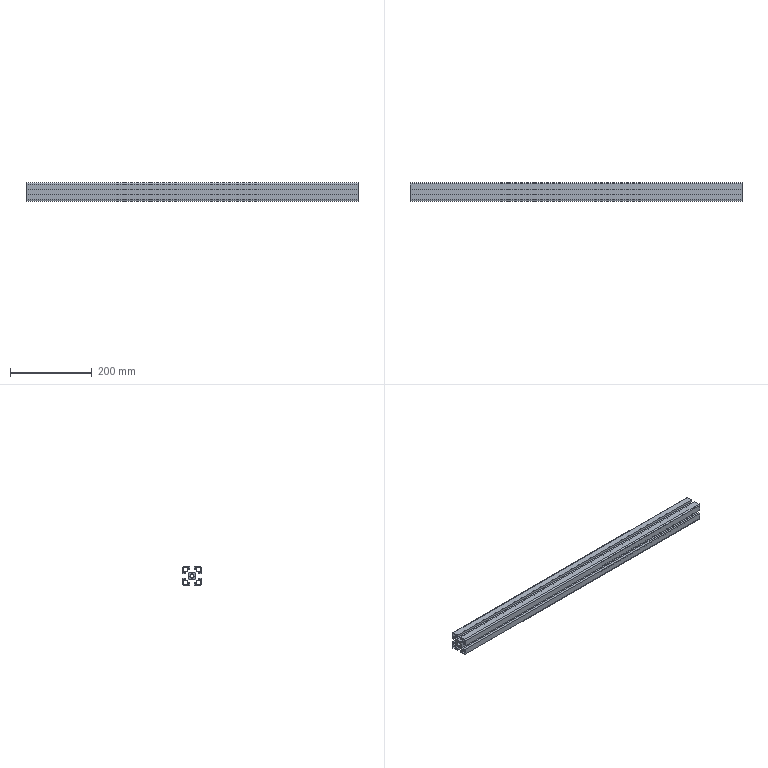Part | STEP file | 1_3 | 1 solid | 87 faces | box 810 x 45 x 45 mm | volume 662372 mm3 | plane 78 | cylinder 9 | commonest cylinder face diameters 2 x4 6 x4 10 x1